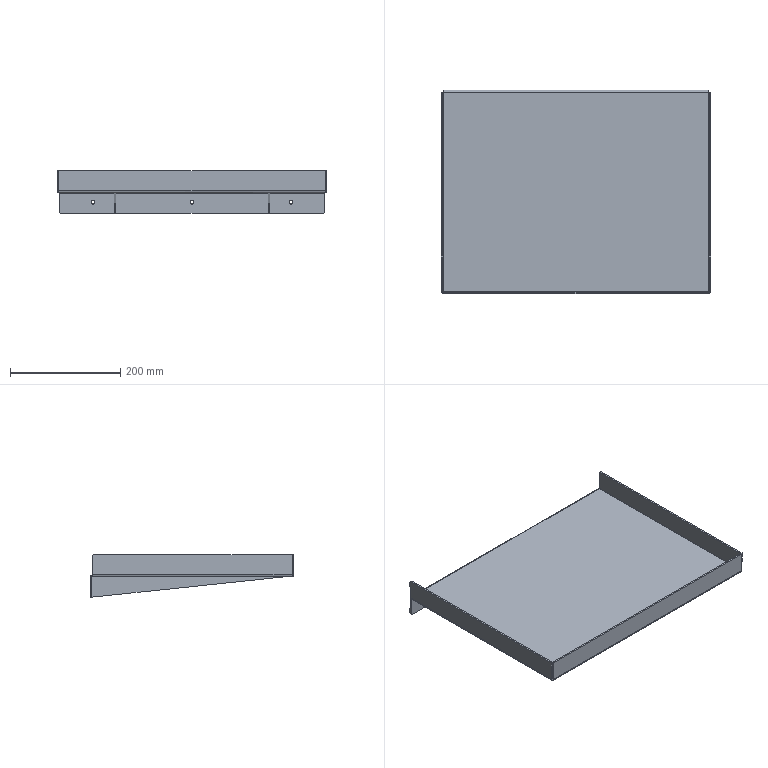Part | SolidWorks | features Gusset 2, EdgeFlange 1, Fillet 1, FlatPattern 1, HoleWzd 1, SMBaseFlange 1, SheetMetal 1 | 3 solids | 58 faces | box 490 x 370 x 77 mm | volume 765884 mm3 | plane 36 | cylinder 18 | spline 4 | commonest cylinder face diameters 7 x10 1 x4 6 x4